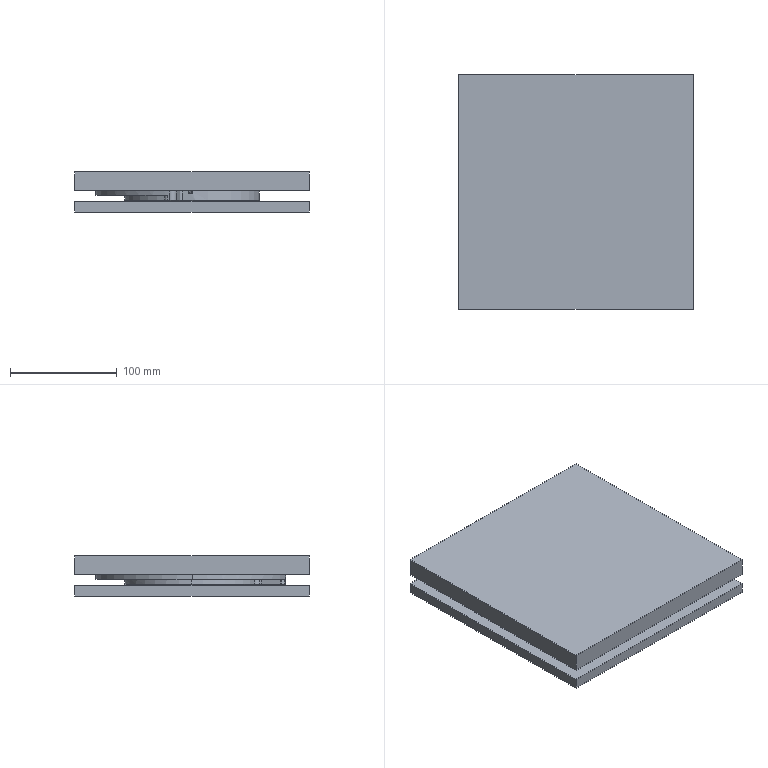NC program | NX | posted with a generic post | part box 220 x 220 x 37.5 mm
Lines 1 to 818 of 4969:
N10 G17 G21 G94 G90
(ADAPTIVE_MILLING_COPY_COPY , TOOL : D10)
N12 T03 M6
N14 G54
N16 G17 G0 G90 X-76.959 Y-29.515 S8000 M3
N18 G43 Z30. H3
N20 Z-4.5
N22 G94 G3 X-76.959 Y-29.515 Z-4.994 I2.51 J-3.735 F1000.
N24 X-76.959 Y-29.515 Z-5.487 I2.51 J-3.735
N26 X-76.959 Y-29.515 Z-5.981 I2.51 J-3.735
N28 X-76.959 Y-29.515 Z-6.474 I2.51 J-3.735
N30 X-76.959 Y-29.515 Z-6.968 I2.51 J-3.735
N32 X-76.959 Y-29.515 Z-7.461 I2.51 J-3.735
N34 X-76.959 Y-29.515 Z-7.955 I2.51 J-3.735
N36 X-76.959 Y-29.515 Z-8.448 I2.51 J-3.735
N38 X-76.959 Y-29.515 Z-8.942 I2.51 J-3.735
N40 X-76.959 Y-29.515 Z-9.435 I2.51 J-3.735
N42 X-76.959 Y-29.515 Z-9.929 I2.51 J-3.735
N44 X-76.959 Y-29.515 Z-10.422 I2.51 J-3.735
N46 X-76.959 Y-29.515 Z-10.916 I2.51 J-3.735
N48 X-76.959 Y-29.515 Z-11.409 I2.51 J-3.735
N50 X-76.959 Y-29.515 Z-11.903 I2.51 J-3.735
N52 X-74.448 Y-28.75 Z-12.35 R-4.5
N54 X-71.843 Y-29.571 R-4.501 F3500.
N56 X-79.316 Y-34.242 R4.669
N58 X-70.976 Y-29.663 R-4.977
N60 X-79.544 Y-35.212 R5.197
N62 X-70.592 Y-29.324 R-5.476
N64 X-80.049 Y-35.338 R5.713
N66 X-69.779 Y-29.447 R-5.996
N68 X-80.555 Y-35.529 R6.255
N70 X-69.211 Y-29.287 R-6.539
N72 X-81.051 Y-35.798 R6.811
N74 X-68.461 Y-29.383 R-7.099
N76 X-81.371 Y-36.522 R7.387
N78 X-67.943 Y-29.096 R-7.686
N80 X-82.268 Y-35.885 R7.977
N82 X-66.893 Y-29.789 R-8.279
N84 X-82.846 Y-36.084 R8.584
N86 X-66.106 Y-30.082 R-8.893
N88 X-83.638 Y-35.591 R9.201
N90 X-65.246 Y-30.689 R-9.518
N92 X-84.379 Y-35.214 R9.837
N94 X-64.383 Y-31.629 R10.159
N96 X-85.001 Y-35.455 R-10.488
N98 X-63.728 Y-31.519 R10.82
N100 X-85.867 Y-34.038 R11.152
N102 X-62.972 Y-32.124 R-11.489
N104 X-86.567 Y-33.269 R11.826
N106 X-62.238 Y-33.484 R12.165
N108 X-87.215 Y-32.245 R12.51
N110 X-61.613 Y-34.613 R12.856
N112 X-85.285 Y-25.329 R13.185
N114 X-87.451 Y-37.11 R13.203
N116 X-85.584 Y-40.924 R36.55
N118 X-69.729 Y-46.031 R13.403
N120 X-65.769 Y-43.648 R45.627
N122 X-61.177 Y-29.971 R13.404
N124 G2 X-62.905 Y-26.146 R61.413
N126 G3 X-71.532 Y-19.668 R12.951
N128 X-88.733 Y-33.803 R14.043
N130 G1 X-87.469 Y-37.067
N132 X-86.14 Y-39.947
N134 G3 X-84.694 Y-42.852 R21.488
N136 X-78.233 Y-47.097 R11.843
N138 X-72.577 Y-47.493 R14.192
N140 X-69.664 Y-45.994 R22.521
N142 X-69.806 Y-44.984 R0.551
N144 G1 X-70.024 Y-44.93
N146 X-71.965 Y-44.448 Z-12.25
N148 X-82.409 Y-41.859
N150 X-84.351 Y-41.378 Z-12.35
N152 G3 X-84.937 Y-41.406 R0.694
N154 X-85.144 Y-42.102 R0.554
N156 X-77.927 Y-47.901 R10.278
N158 X-72.58 Y-47.494 R10.689
N160 G1 X-72.466 Y-47.441
N162 G3 X-72.585 Y-46.404 R0.55
N164 G1 X-82.495 Y-44.345
N166 G3 X-82.929 Y-45.264 R0.551
N168 G1 X-82.791 Y-45.417
N170 X-82.716 Y-45.486
N172 X-81.828 Y-46.165
N174 G3 X-79.182 Y-47.535 R8.747
N176 G1 X-77.927 Y-47.901
N178 X-77.029 Y-48.003
N180 X-76.13 Y-48.091
N182 X-75.228 Y-48.03
N184 X-74.328 Y-47.953
N186 X-73.452 Y-47.731
N188 X-72.58 Y-47.494
N190 X-70.963 Y-46.744
N192 X-66.698 Y-44.281
N194 G3 X-63.932 Y-42.583 R22.347
N196 X-60.357 Y-36.135 R11.686
N198 X-60.112 Y-32.012 R13.658
N200 G1 X-61.211 Y-29.907
N202 G3 X-62.231 Y-30.024 R0.551
N204 G1 X-62.301 Y-30.296
N206 X-62.801 Y-32.232 Z-12.25
N208 X-64.895 Y-40.336
N210 X-65.395 Y-42.272 Z-12.35
N212 X-65.452 Y-42.501
N214 X-65.453 Y-42.736
N216 G3 X-64.641 Y-43.094 R0.551
N218 X-62.357 Y-41.58 R10.606
N220 X-59.502 Y-35.576 R11.215
N222 X-59.353 Y-33.465 R6.671
N224 G1 X-60.163 Y-31.914
N226 G3 X-61.178 Y-32.012 R0.551
N228 G1 X-61.239 Y-32.218
N230 X-61.808 Y-34.135 Z-12.25
N232 X-63.389 Y-39.468
N234 X-63.958 Y-41.386 Z-12.35
N236 X-64.023 Y-41.6
N238 X-64.058 Y-41.821
N240 G3 X-63.234 Y-42.281 R0.551
N242 X-61.017 Y-40.685 R7.564
N244 X-58.687 Y-34.729 R10.602
N246 X-59.189 Y-33.779 R2.823
N248 G1 X-59.363 Y-33.447
N250 G3 X-60.372 Y-33.527 R0.551
N252 G1 X-62.861 Y-41.03
N254 G3 X-62.043 Y-41.594 R0.551
N256 X-58.813 Y-38.102 R6.347
N258 X-58.176 Y-35.454 R5.89
N260 G1 X-58.211 Y-35.353
N262 X-58.805 Y-34.398
N264 G3 X-59.791 Y-34.505 R0.551
N266 G1 X-61.885 Y-40.458
N268 G3 X-61.068 Y-41.031 R0.551
N270 X-57.698 Y-36.382 R5.887
N272 G1 X-57.705 Y-36.258
N274 X-57.736 Y-36.137
N276 X-57.752 Y-36.091
N278 X-58.214 Y-35.348
N280 G3 X-59.194 Y-35.44 R0.551
N282 G1 X-60.908 Y-39.88
N284 G3 X-60.094 Y-40.469 R0.551
N286 X-57.388 Y-37.376 R4.939
N288 X-57.38 Y-36.689 R1.267
N290 G1 X-57.776 Y-36.052
N292 G3 X-58.754 Y-36.139 R0.551
N294 G1 X-60.04 Y-39.375
N296 G3 X-59.228 Y-39.969 R0.551
N298 X-57.418 Y-38.484 R4.401
N300 X-57.076 Y-37.193 R1.664
N302 G1 X-57.087 Y-37.161
N304 X-57.417 Y-36.63
N306 G3 X-58.401 Y-36.733 R0.551
N308 G1 X-59.178 Y-38.891
N310 G3 X-58.362 Y-39.469 R0.551
N312 X-56.922 Y-38.148 R2.881
N314 X-56.88 Y-37.494 R0.883
N316 G1 X-57.144 Y-37.07
N318 G3 X-58.138 Y-37.202 R0.551
N320 G1 X-58.533 Y-38.545
N322 G3 X-57.713 Y-39.094 R0.551
N324 X-56.699 Y-38.062 R1.712
N326 X-56.884 Y-37.487 R0.874
N328 X-57.871 Y-37.598 R0.551
N330 G1 X-58.097 Y-38.274
N332 G3 X-57.28 Y-38.844 R0.551
N334 X-56.62 Y-38.151 R1.03
N336 X-56.807 Y-37.612 R0.903
N338 X-57.817 Y-37.988 R0.55
N340 G1 X-57.783 Y-38.214
N342 X-57.718 Y-38.434
N344 G3 X-56.955 Y-38.656 R0.552
N346 X-56.662 Y-37.852 R0.583
N348 G1 X-59.189 Y-33.779
N350 X-61.558 Y-29.24
N352 X-62.743 Y-26.484
N354 G3 X-64.114 Y-23.548 R20.329
N356 X-70.254 Y-19.25 R11.851
N358 X-89.427 Y-31.954 R14.762
N360 G1 X-89.413 Y-32.044
N362 X-88.691 Y-33.91
N364 G3 X-88.036 Y-34.242 R0.554
N366 G1 X-86.162 Y-33.545 Z-12.25
N368 X-65.722 Y-25.908
N370 X-63.85 Y-25.205 Z-12.35
N372 G3 X-63.579 Y-24.536 R0.554
N374 X-64.724 Y-22.056 R7.534
N376 X-70.555 Y-18.382 R11.483
N378 X-89.96 Y-30.336 R15.473
N380 X-89.408 Y-32.059 R9.865
N382 X-88.751 Y-32.391 R0.554
N384 G1 X-86.861 Y-31.737 Z-12.25
N386 X-66.218 Y-24.576
N388 X-64.329 Y-23.92 Z-12.35
N390 G3 X-64.026 Y-23.236 R0.553
N392 X-66.919 Y-19.308 R6.494
N394 X-77.582 Y-17.26 R14.577
N396 X-90.396 Y-28.882 R16.145
N398 G1 X-90.399 Y-29.007
N400 X-90.394 Y-29.071
N402 X-89.942 Y-30.502
N404 G3 X-89.31 Y-30.876 R0.554
N406 G1 X-87.407 Y-30.26 Z-12.25
N408 X-66.596 Y-23.478
N410 X-64.696 Y-22.856 Z-12.35
N412 G3 X-64.392 Y-22.172 R0.553
N414 X-67.237 Y-18.369 R6.139
N416 X-76.833 Y-16.363 R14.504
N418 X-90.71 Y-27.344 R16.839
N420 X-90.781 Y-27.843 R3.366
N422 G1 X-90.367 Y-29.154
N424 G3 X-89.735 Y-29.528 R0.554
N426 G1 X-87.826 Y-28.933 Z-12.25
N428 X-66.969 Y-22.393
N430 X-65.061 Y-21.792 Z-12.35
N432 G3 X-64.757 Y-21.108 R0.553
N434 X-67.471 Y-17.513 R5.788
N436 X-75.969 Y-15.503 R14.213
N438 X-90.942 Y-25.844 R17.566
N440 X-91.142 Y-26.701 R2.262
N442 G1 X-90.765 Y-27.893
N444 G3 X-90.132 Y-28.267 R0.554
N446 G1 X-88.216 Y-27.695 Z-12.25
N448 X-67.302 Y-21.424
N450 X-65.387 Y-20.847 Z-12.35
N452 G3 X-65.082 Y-20.162 R0.553
N454 X-65.867 Y-18.343 R5.932
N456 X-70.182 Y-15.489 R8.932
N458 X-82.83 Y-16.479 R17.009
N460 X-91.201 Y-24.596 R17.861
N462 X-91.463 Y-25.68 R1.818
N464 G1 X-91.453 Y-25.714
N466 X-91.114 Y-26.787
N468 G3 X-90.48 Y-27.161 R0.554
N470 G1 X-88.556 Y-26.616 Z-12.25
N472 X-67.566 Y-20.654
N474 X-65.643 Y-20.106 Z-12.35
N476 G3 X-65.305 Y-19.452 R0.554
N478 X-67.529 Y-16.117 R4.962
N480 X-74.724 Y-13.937 R13.125
N482 X-91.36 Y-23.252 R18.728
N484 X-91.774 Y-24.419 R2.696
N486 G1 X-91.474 Y-25.633
N488 G3 X-90.834 Y-26.04 R0.553
N490 G1 X-88.903 Y-25.517 Z-12.25
N492 X-67.811 Y-19.79
N494 X-65.881 Y-19.265 Z-12.35
N496 G3 X-65.527 Y-18.605 R0.553
N498 X-67.766 Y-15.284 R4.928
N500 X-74.979 Y-13.159 R13.186
N502 X-91.477 Y-21.932 R19.338
N504 X-92.044 Y-23.326 R3.132
N506 G1 X-91.744 Y-24.54
N508 G3 X-91.137 Y-24.953 R0.554
N510 G1 X-89.201 Y-24.452 Z-12.25
N512 X-68.037 Y-18.925
N514 X-66.102 Y-18.418 Z-12.35
N516 G3 X-65.748 Y-17.759 R0.553
N518 X-68.01 Y-14.456 R4.877
N520 X-74.987 Y-12.385 R13.087
N522 X-91.623 Y-20.742 R19.839
N524 X-92.304 Y-22.204 R4.269
N526 G1 X-92.302 Y-22.279
N528 X-92.033 Y-23.372
N530 G3 X-91.425 Y-23.785 R0.554
N532 G1 X-89.483 Y-23.307 Z-12.25
N534 X-68.264 Y-18.054
N536 X-66.324 Y-17.572 Z-12.35
N538 G3 X-65.969 Y-16.912 R0.553
N540 X-68.152 Y-13.698 R4.798
N542 X-75.122 Y-11.611 R12.998
N544 X-91.598 Y-19.365 R20.468
N546 X-92.55 Y-21.111 R5.955
N548 X-92.284 Y-22.355 R6.523
N550 X-91.676 Y-22.768 R0.554
N552 G1 X-89.731 Y-22.303 Z-12.25
N554 X-68.489 Y-17.195
N556 X-66.545 Y-16.725 Z-12.35
N558 G3 X-66.191 Y-16.066 R0.553
N560 X-68.3 Y-12.945 R4.716
N562 X-74.762 Y-10.859 R12.562
N564 X-91.767 Y-18.315 R20.807
N566 X-92.797 Y-20.154 R5.347
N568 X-92.526 Y-21.374 R35.32
N570 X-91.918 Y-21.787 R0.554
N572 G1 X-89.968 Y-21.342 Z-12.25
N574 X-68.684 Y-16.451
N576 X-66.735 Y-16. Z-12.35
N578 G3 X-66.38 Y-15.34 R0.553
N580 X-68.439 Y-12.195 R4.628
N582 X-74.891 Y-10.083 R12.549
N584 X-91.999 Y-17.359 R21.134
N586 X-93.008 Y-19.073 R5.965
N588 X-92.783 Y-20.334 R5.638
N590 X-92.174 Y-20.747 R0.554
N592 G1 X-90.219 Y-20.323 Z-12.25
N594 X-68.888 Y-15.669
N596 X-66.935 Y-15.241 Z-12.35
N598 G3 X-66.559 Y-14.617 R0.554
N600 X-68.367 Y-11.601 R4.275
N602 X-74.385 Y-9.367 R11.921
N604 X-87.846 Y-12.695 R21.193
N606 X-92.728 Y-17.108 R16.692
N608 X-93.207 Y-18.169 R2.453
N610 G1 X-93.007 Y-19.276
N612 G3 X-92.425 Y-19.727 R0.554
N614 G1 X-90.466 Y-19.328 Z-12.25
N616 X-69.056 Y-14.915
N618 X-67.097 Y-14.511 Z-12.35
N620 G3 X-66.694 Y-13.88 R0.553
N622 X-68.493 Y-10.856 R4.293
N624 X-74.376 Y-8.61 R11.794
N626 X-87.35 Y-11.424 R21.302
N628 X-92.793 Y-15.945 R17.496
N630 X-93.388 Y-17.165 R2.508
N632 G1 X-93.188 Y-18.272
N634 G3 X-92.609 Y-18.723 R0.554
N636 G1 X-90.645 Y-18.344 Z-12.25
N638 X-69.194 Y-14.157
N640 X-67.231 Y-13.773 Z-12.35
N642 G3 X-66.828 Y-13.142 R0.553
N644 X-68.611 Y-10.107 R4.318
N646 X-74.733 Y-7.804 R12.003
N648 X-88.032 Y-10.85 R21.836
N650 X-93.061 Y-15.094 R16.446
N652 X-93.567 Y-16.172 R2.304
N654 G1 X-93.367 Y-17.279
N656 G3 X-92.788 Y-17.73 R0.554
N658 G1 X-90.82 Y-17.37 Z-12.25
N660 X-69.332 Y-13.4
N662 X-67.366 Y-13.035 Z-12.35
N664 G3 X-66.963 Y-12.404 R0.553
N666 X-68.827 Y-9.282 R4.373
N668 X-75.089 Y-7. R12.255
N670 X-88.063 Y-9.897 R22.221
N672 X-93.097 Y-13.945 R16.752
N674 X-93.743 Y-15.199 R2.616
N676 G1 X-93.565 Y-16.183
N678 G3 X-92.985 Y-16.634 R0.554
N680 G1 X-91.013 Y-16.301 Z-12.25
N682 X-69.472 Y-12.635
N684 X-67.5 Y-12.297 Z-12.35
N686 G3 X-67.098 Y-11.666 R0.553
N688 X-68.947 Y-8.533 R4.412
N690 X-74.949 Y-6.248 R12.117
N692 X-87.536 Y-8.66 R22.256
N694 X-93.118 Y-12.808 R17.79
N696 X-93.914 Y-14.203 R3.167
N698 G1 X-93.915 Y-14.242
N700 X-93.738 Y-15.226
N702 G3 X-93.157 Y-15.677 R0.554
N704 G1 X-91.182 Y-15.361 Z-12.25
N706 X-69.609 Y-11.88
N708 X-67.635 Y-11.559 Z-12.35
N710 G3 X-67.232 Y-10.928 R0.553
N712 X-69.064 Y-7.785 R4.412
N714 X-75.178 Y-5.453 R12.178
N716 X-87.888 Y-7.892 R22.628
N718 X-93.364 Y-11.971 R17.075
N720 X-94.059 Y-13.197 R2.821
N722 G1 X-93.982 Y-13.868
N724 X-93.977 Y-13.903
N726 X-93.91 Y-14.272
N728 G3 X-93.328 Y-14.723 R0.554
N730 G1 X-91.351 Y-14.423 Z-12.25
N732 X-69.747 Y-11.126
N734 X-67.77 Y-10.822 Z-12.35
N736 G3 X-67.367 Y-10.19 R0.553
N738 X-69.074 Y-7.12 R4.279
N740 X-75.022 Y-4.706 R11.95
N742 X-87.211 Y-6.636 R22.517
N744 X-93.277 Y-10.745 R18.617
N746 X-94.167 Y-12.088 R4.189
N748 G1 X-94.177 Y-12.177
N750 X-94.048 Y-13.295
N752 G3 X-93.498 Y-13.782 R0.554
N754 G1 X-91.517 Y-13.507 Z-12.25
N756 X-69.871 Y-10.454
N758 X-67.891 Y-10.173 Z-12.35
N760 G3 X-67.468 Y-9.579 R0.554
N762 X-68.981 Y-6.542 R4.073
N764 X-74.733 Y-3.989 R11.493
N766 X-86.734 Y-5.514 R22.321
N768 X-93.33 Y-9.712 R19.103
N770 X-94.287 Y-11.152 R3.369
N772 G1 X-94.291 Y-11.187
N774 X-94.177 Y-12.18
N776 G3 X-93.627 Y-12.667 R0.554
N778 G1 X-91.642 Y-12.42 Z-12.25
N780 X-69.981 Y-9.684
N782 X-67.997 Y-9.433 Z-12.35
N784 G3 X-67.547 Y-8.833 R0.553
N786 X-69.068 Y-5.798 R4.118
N788 X-74.561 Y-3.26 R11.361
N790 X-86.354 Y-4.459 R22.14
N792 X-93.197 Y-8.502 R20.134
N794 X-94.386 Y-10.09 R5.034
N796 X-94.288 Y-11.215 R14.31
N798 X-93.738 Y-11.702 R0.554
N800 G1 X-91.75 Y-11.481 Z-12.25
N802 X-70.049 Y-9.036
N804 X-68.062 Y-8.811 Z-12.35
N806 G3 X-67.613 Y-8.212 R0.553
N808 X-69.241 Y-4.965 R4.289
N810 X-74.998 Y-2.413 R11.816
N812 X-87.251 Y-3.9 R22.68
N814 X-93.492 Y-7.74 R18.787
N816 X-94.501 Y-9.151 R4.324
N818 G1 X-94.513 Y-9.261
N820 X-94.399 Y-10.254
N822 G3 X-93.848 Y-10.741 R0.554
N824 G1 X-91.859 Y-10.536 Z-12.25
N826 X-70.13 Y-8.274
N828 X-68.141 Y-8.065 Z-12.35
N830 G3 X-67.692 Y-7.466 R0.553
N832 X-69.317 Y-4.217 R4.3
N834 X-75.061 Y-1.633 R11.874
N836 X-86.978 Y-2.885 R22.734
N838 X-93.512 Y-6.715 R19.066
N840 X-94.612 Y-8.211 R4.22
N842 G1 X-94.623 Y-8.309
N844 X-94.509 Y-9.303
N846 G3 X-93.957 Y-9.79 R0.554
N848 G1 X-91.966 Y-9.6 Z-12.25
N850 X-70.21 Y-7.512
N852 X-68.22 Y-7.319 Z-12.35
N854 G3 X-67.771 Y-6.72 R0.553
N856 X-69.391 Y-3.467 R4.323
N858 X-75.244 Y-0.828 R12.04
N860 X-87.635 Y-2.228 R23.143
N862 X-93.793 Y-5.958 R17.855
N864 X-94.703 Y-7.286 R2.976
N866 G1 X-94.673 Y-7.865
N868 X-94.67 Y-7.901
N870 X-94.613 Y-8.398
N872 G3 X-94.061 Y-8.885 R0.554
N874 G1 X-92.069 Y-8.708 Z-12.25
N876 X-70.291 Y-6.754
N878 X-68.299 Y-6.573 Z-12.35
N880 G3 X-67.85 Y-5.974 R0.553
N882 X-69.462 Y-2.717 R4.335
N884 X-75.3 Y-0.045 R12.025
N886 X-87.587 Y-1.299 R23.226
N888 X-93.803 Y-4.936 R18.29
N890 X-94.755 Y-6.266 R3.047
N892 G1 X-94.698 Y-7.39
N894 G3 X-94.174 Y-7.911 R0.554
N896 G1 X-92.18 Y-7.754 Z-12.25
N898 X-70.372 Y-5.992
N900 X-68.379 Y-5.828 Z-12.35
N902 G3 X-67.929 Y-5.229 R0.553
N904 X-69.521 Y-1.966 R4.338
N906 X-75.223 Y0.714 R12.051
N908 X-87.643 Y-0.417 R23.247
N910 X-93.799 Y-3.913 R18.278
N912 X-94.789 Y-5.185 R4.096
N914 G1 X-94.806 Y-5.28
N916 X-94.755 Y-6.279
N918 G3 X-94.237 Y-6.8 R0.554
N920 G1 X-92.241 Y-6.678 Z-12.25
N922 X-70.445 Y-5.3
N924 X-68.45 Y-5.171 Z-12.35
N926 G3 X-67.993 Y-4.612 R0.554
N928 X-69.297 Y-1.484 R3.993
N930 X-74.643 Y1.351 R11.33
N932 X-86.132 Y0.961 R22.475
N934 X-93.491 Y-2.641 R20.316
N936 X-94.812 Y-4.126 R5.666
N938 X-94.805 Y-5.304 R4.11
N940 X-94.287 Y-5.825 R0.554
N942 G1 X-92.29 Y-5.719 Z-12.25
N944 X-70.506 Y-4.535
N946 X-68.509 Y-4.426 Z-12.35
N948 G3 X-68.016 Y-3.862 R0.553
N950 X-69.336 Y-0.736 R4.081
N952 X-74.787 Y2.161 R11.508
N954 X-86.16 Y1.836 R22.684
N956 X-93.55 Y-1.704 R20.399
N958 X-94.867 Y-3.189 R5.242
N960 X-94.854 Y-4.351 R4.711
N962 X-94.335 Y-4.871 R0.554
N964 G1 X-92.337 Y-4.791 Z-12.25
N966 X-70.526 Y-3.885
N968 X-68.527 Y-3.801 Z-12.35
N970 G3 X-68.035 Y-3.238 R0.553
N972 X-69.368 Y0.01 R4.144
N974 X-75.166 Y3.031 R11.827
N976 X-87.26 Y2.401 R23.356
N978 X-93.789 Y-0.925 R18.764
N980 X-94.918 Y-2.248 R4.993
N982 X-94.902 Y-3.403 R5.053
N984 X-94.383 Y-3.924 R0.554
N986 G1 X-92.384 Y-3.859 Z-12.25
N988 X-70.549 Y-3.121
N990 X-68.55 Y-3.052 Z-12.35
N992 G3 X-68.058 Y-2.488 R0.553
N994 X-69.394 Y0.761 R4.194
N996 X-74.934 Y3.754 R11.757
N998 X-86.555 Y3.49 R23.128
N1000 X-93.735 Y0.09 R19.519
N1002 X-94.958 Y-1.31 R4.498
N1004 X-94.949 Y-2.491 R33.287
N1006 X-94.429 Y-3.012 R0.554
N1008 G1 X-92.43 Y-2.959 Z-12.25
N1010 X-70.572 Y-2.359
N1012 X-68.573 Y-2.302 Z-12.35
N1014 G3 X-68.08 Y-1.738 R0.553
N1016 X-69.418 Y1.512 R4.231
N1018 X-74.941 Y4.537 R11.816
N1020 X-86.686 Y4.334 R23.211
N1022 X-93.672 Y1.099 R19.356
N1024 X-94.935 Y-0.267 R4.893
N1026 G1 X-94.964 Y-0.387
N1028 X-94.976 Y-1.387
N1030 G3 X-94.484 Y-1.94 R0.554
N1032 G1 X-92.485 Y-1.914 Z-12.25
N1034 X-70.596 Y-1.585
N1036 X-68.597 Y-1.553 Z-12.35
N1038 G3 X-68.103 Y-0.989 R0.553
N1040 X-69.437 Y2.265 R4.248
N1042 X-75.064 Y5.354 R11.959
N1044 X-86.811 Y5.181 R23.424
N1046 X-93.702 Y2.033 R19.314
N1048 X-94.94 Y0.654 R3.704
N1050 G1 X-94.952 Y0.606
N1052 X-94.964 Y-0.394
N1054 G3 X-94.48 Y-0.946 R0.554
N1056 G1 X-92.481 Y-0.939 Z-12.25
N1058 X-70.62 Y-0.817
N1060 X-68.62 Y-0.803 Z-12.35
N1062 G3 X-68.126 Y-0.239 R0.553
N1064 X-69.439 Y3.005 R4.238
N1066 X-74.924 Y6.1 R11.875
N1068 X-86.671 Y6.094 R23.317
N1070 X-93.709 Y2.974 R19.204
N1072 X-94.903 Y1.712 R4.728
N1074 X-94.952 Y0.577 R8.175
N1076 X-94.468 Y0.024 R0.554
N1078 G1 X-92.468 Y0.016 Z-12.25
N1080 X-70.643 Y-0.029
N1082 X-68.644 Y-0.03 Z-12.35
N1084 G3 X-68.148 Y0.493 R0.554
N1086 X-69.19 Y3.47 R3.847
N1088 X-74.188 Y6.656 R11.132
N1090 X-85.304 Y7.253 R22.457
N1092 X-93.308 Y4.205 R20.969
N1094 X-94.9 Y2.644 R5.076
N1096 G1 X-94.928 Y2.526
N1098 X-94.94 Y1.526
N1100 G3 X-94.456 Y0.974 R0.554
N1102 G1 X-92.457 Y0.932 Z-12.25
N1104 X-70.658 Y0.506
N1106 X-68.658 Y0.467 Z-12.35
N1108 G3 X-68.126 Y0.992 R0.553
N1110 X-69.176 Y4.216 R4.005
N1112 X-74.392 Y7.513 R11.367
N1114 X-85.759 Y8.03 R22.8
N1116 X-93.4 Y5.07 R20.315
N1118 X-94.89 Y3.585 R4.699
N1120 G1 X-94.916 Y3.476
N1122 X-94.929 Y2.476
N1124 G3 X-94.444 Y1.923 R0.554
N1126 G1 X-92.445 Y1.866 Z-12.25
N1128 X-70.625 Y1.27
N1130 X-68.626 Y1.216 Z-12.35
N1132 G3 X-68.092 Y1.742 R0.553
N1134 X-69.235 Y5.06 R4.127
N1136 X-74.472 Y8.331 R11.625
N1138 X-86.085 Y8.834 R23.081
N1140 X-93.483 Y5.936 R19.777
N1142 X-94.872 Y4.525 R4.148
N1144 G1 X-94.886 Y4.48
N1146 X-94.906 Y4.21
N1148 X-94.908 Y4.174
N1150 X-94.917 Y3.424
N1152 G3 X-94.431 Y2.871 R0.554
N1154 G1 X-92.433 Y2.79 Z-12.25
N1156 X-70.596 Y1.919
N1158 X-68.598 Y1.841 Z-12.35
N1160 G3 X-68.064 Y2.366 R0.553
N1162 X-69.209 Y5.809 R4.222
N1164 X-74.546 Y9.151 R11.817
N1166 X-86.527 Y9.614 R23.401
N1168 X-93.456 Y6.868 R19.223
N1170 X-94.785 Y5.57 R4.335
N1172 G1 X-94.809 Y5.492
N1174 X-94.894 Y4.37
N1176 G3 X-94.421 Y3.784 R0.553
N1178 G1 X-92.423 Y3.689 Z-12.25
N1180 X-70.563 Y2.681
N1182 X-68.565 Y2.59 Z-12.35
N1184 G3 X-68.031 Y3.115 R0.553
N1186 X-69.177 Y6.559 R4.254
N1188 X-74.496 Y9.933 R11.925
N1190 X-86.596 Y10.47 R23.563
N1192 X-93.421 Y7.801 R18.893
N1194 X-94.686 Y6.609 R4.91
N1196 X-94.81 Y5.475 R6.781
N1198 X-94.362 Y4.892 R0.554
N1200 G1 X-92.366 Y4.768 Z-12.25
N1202 X-70.528 Y3.457
N1204 X-68.531 Y3.339 Z-12.35
N1206 G3 X-67.997 Y3.864 R0.553
N1208 X-69.142 Y7.311 R4.285
N1210 X-74.56 Y10.757 R12.061
N1212 X-87.028 Y11.246 R23.752
N1214 X-93.588 Y8.588 R17.905
N1216 X-94.633 Y7.53 R3.756
N1218 G1 X-94.66 Y7.441
N1220 X-94.736 Y6.444
N1222 G3 X-94.289 Y5.861 R0.554
N1224 G1 X-92.294 Y5.721 Z-12.25
N1226 X-70.493 Y4.223
N1228 X-68.498 Y4.089 Z-12.35
N1230 G3 X-67.963 Y4.614 R0.553
N1232 X-69.104 Y8.063 R4.311
N1234 X-74.384 Y11.501 R12.08
N1236 X-86.721 Y12.179 R23.716
N1238 X-93.336 Y9.657 R18.089
N1240 X-94.572 Y8.447 R3.425
N1242 G1 X-94.588 Y8.397
N1244 X-94.663 Y7.4
N1246 G3 X-94.215 Y6.817 R0.554
N1248 G1 X-92.222 Y6.661 Z-12.25
N1250 X-70.459 Y4.988
N1252 X-68.465 Y4.838 Z-12.35
N1254 G3 X-67.93 Y5.363 R0.553
N1256 X-68.827 Y8.521 R4.033
N1258 X-73.969 Y12.151 R11.517
N1260 X-85.542 Y13.243 R23.148
N1262 X-92.971 Y10.791 R19.825
N1264 X-94.465 Y9.485 R4.993
N1266 X-94.591 Y8.345 R5.919
N1268 X-94.143 Y7.763 R0.554
N1270 G1 X-92.152 Y7.576 Z-12.25
N1272 X-70.433 Y5.567
N1274 X-68.441 Y5.384 Z-12.35
N1276 G3 X-67.888 Y5.868 R0.554
N1278 X-68.688 Y9.163 R4.013
N1280 X-73.649 Y12.832 R11.337
N1282 X-84.948 Y14.177 R22.897
N1284 X-92.787 Y11.79 R20.404
N1286 X-94.392 Y10.423 R5.232
N1288 X-94.517 Y9.326 R6.795
N1290 X-94.067 Y8.744 R0.554
N1292 G1 X-92.078 Y8.54 Z-12.25
N1294 X-70.359 Y6.331
N1296 X-68.369 Y6.129 Z-12.35
N1298 G3 X-67.798 Y6.613 R0.553
N1300 X-68.612 Y9.906 R4.06
N1302 X-73.553 Y13.604 R11.417
N1304 X-84.717 Y15.058 R22.841
N1306 X-92.589 Y12.782 R20.547
N1308 X-94.235 Y11.462 R5.694
N1310 X-94.447 Y10.235 R6.787
N1312 X-94. Y9.635 R0.553
N1314 G1 X-92.011 Y9.42 Z-12.25
N1316 X-70.268 Y7.086
N1318 X-68.279 Y6.874 Z-12.35
N1320 G3 X-67.708 Y7.358 R0.553
N1322 X-68.53 Y10.651 R4.101
N1324 X-73.452 Y14.378 R11.496
N1326 X-84.976 Y15.885 R23.01
N1328 X-92.492 Y13.709 R20.027
N1330 X-94.126 Y12.384 R4.54
N1332 G1 X-94.155 Y12.306
N1334 X-94.295 Y11.316
N1336 G3 X-93.885 Y10.706 R0.554
N1338 G1 X-91.901 Y10.454 Z-12.25
N1340 X-70.19 Y7.741
N1342 X-68.205 Y7.494 Z-12.35
N1344 G3 X-67.633 Y7.978 R0.553
N1346 X-68.515 Y11.5 R4.261
N1348 X-73.459 Y15.202 R11.757
N1350 X-85.106 Y16.726 R23.23
N1352 X-92.499 Y14.577 R19.631
N1354 X-93.956 Y13.416 R5.194
N1356 X-94.159 Y12.279 R5.061
N1358 X-93.75 Y11.669 R0.554
N1360 G1 X-91.768 Y11.4 Z-12.25
N1362 X-70.098 Y8.502
N1364 X-68.115 Y8.239 Z-12.35
N1366 G3 X-67.543 Y8.723 R0.553
N1368 X-68.423 Y12.246 R4.294
N1370 X-73.575 Y16.079 R12.057
N1372 X-85.603 Y17.523 R23.677
N1374 X-92.604 Y15.372 R18.187
N1376 X-93.84 Y14.336 R4.217
N1378 X-94.026 Y13.225 R23.169
N1380 X-93.616 Y12.616 R0.554
N1382 G1 X-91.637 Y12.332 Z-12.25
N1384 X-70.006 Y9.262
N1386 X-68.026 Y8.984 Z-12.35
N1388 G3 X-67.454 Y9.467 R0.553
N1390 X-68.329 Y12.993 R4.312
N1392 X-73.459 Y16.856 R12.088
N1394 X-85.351 Y18.411 R23.703
N1396 X-92.491 Y16.295 R18.229
N1398 X-93.719 Y15.253 R3.876
N1400 G1 X-93.755 Y15.158
N1402 X-93.894 Y14.168
N1404 G3 X-93.484 Y13.558 R0.554
N1406 G1 X-91.506 Y13.259 Z-12.25
N1408 X-69.914 Y10.022
N1410 X-67.936 Y9.728 Z-12.35
N1412 G3 X-67.364 Y10.212 R0.553
N1414 X-68.154 Y13.63 R4.203
N1416 X-73.216 Y17.579 R11.949
N1418 X-84.961 Y19.305 R23.583
N1420 X-92.148 Y17.343 R18.744
N1422 X-93.591 Y16.176 R4.038
N1424 G1 X-93.624 Y16.088
N1426 X-93.763 Y15.097
N1428 G3 X-93.352 Y14.487 R0.554
N1430 G1 X-91.378 Y14.167 Z-12.25
N1432 X-69.833 Y10.699
N1434 X-67.858 Y10.383 Z-12.35
N1436 G3 X-67.28 Y10.826 R0.554
N1438 X-67.832 Y14.051 R3.931
N1440 X-72.508 Y18.077 R11.345
N1442 X-83.554 Y20.25 R22.82
N1444 X-91.672 Y18.443 R20.356
N1446 X-93.379 Y17.209 R5.004
N1448 G1 X-93.419 Y17.121
N1450 X-93.605 Y16.218
N1452 X-93.611 Y16.182
N1454 X-93.628 Y16.059
N1456 G3 X-93.216 Y15.448 R0.554
N1458 G1 X-91.246 Y15.103 Z-12.25
N1460 X-69.735 Y11.343
N1462 X-67.764 Y10.999 Z-12.35
N1464 G3 X-67.159 Y11.439 R0.553
N1466 X-67.77 Y14.892 R4.086
N1468 X-72.581 Y18.954 R11.703
N1470 X-83.635 Y21.1 R23.128
N1472 X-91.403 Y19.418 R20.278
N1474 X-93.148 Y18.231 R5.556
N1476 X-93.42 Y17.114 R5.556
N1478 X-93.05 Y16.48 R0.554
N1480 G1 X-91.085 Y16.109 Z-12.25
N1482 X-69.586 Y12.101
N1484 X-67.62 Y11.735 Z-12.35
N1486 G3 X-67.014 Y12.175 R0.553
N1488 X-67.572 Y15.522 R4.081
N1490 X-72.423 Y19.721 R11.709
N1492 X-84.085 Y21.93 R23.435
N1494 X-91.579 Y20.172 R19.045
N1496 X-92.977 Y19.145 R4.316
N1498 G1 X-93.022 Y19.045
N1500 X-93.224 Y18.066
N1502 G3 X-92.854 Y17.431 R0.554
N1504 G1 X-90.894 Y17.035 Z-12.25
N1506 X-69.46 Y12.74
N1508 X-67.499 Y12.348 Z-12.35
N1510 G3 X-66.893 Y12.788 R0.553
N1512 X-67.497 Y16.365 R4.229
N1514 X-72.259 Y20.486 R11.784
N1516 X-83.653 Y22.802 R23.422
N1518 X-91.185 Y21.201 R19.65
N1520 X-92.797 Y20.055 R4.066
N1522 G1 X-92.828 Y19.987
N1524 X-93.03 Y19.008
N1526 G3 X-92.66 Y18.373 R0.554
N1528 G1 X-90.703 Y17.961 Z-12.25
N1530 X-69.312 Y13.491
N1532 X-67.354 Y13.084 Z-12.35
N1534 G3 X-66.748 Y13.524 R0.553
N1536 X-67.352 Y17.104 R4.278
N1538 X-71.981 Y21.193 R11.805
N1540 X-83.592 Y23.655 R23.43
N1542 X-91.01 Y22.116 R19.444
N1544 X-92.554 Y21.073 R5.163
N1546 X-92.838 Y19.938 R4.328
N1548 X-92.468 Y19.303 R0.554
N1550 G1 X-90.514 Y18.877 Z-12.25
N1552 X-69.164 Y14.242
N1554 X-67.209 Y13.82 Z-12.35
N1556 G3 X-66.602 Y14.259 R0.553
N1558 X-67.202 Y17.843 R4.309
N1560 X-72.031 Y22.075 R12.038
N1562 X-84.151 Y24.481 R23.786
N1564 X-91.054 Y22.913 R17.967
N1566 X-92.432 Y21.871 R3.179
N1568 G1 X-92.447 Y21.837
N1570 X-92.649 Y20.858
N1572 G3 X-92.278 Y20.223 R0.554
N1574 G1 X-90.327 Y19.782 Z-12.25
N1576 X-69.016 Y14.992
N1578 X-67.064 Y14.556 Z-12.35
N1580 G3 X-66.457 Y14.995 R0.553
N1582 X-67.019 Y18.531 R4.294
N1584 X-71.913 Y22.874 R12.208
N1586 X-84.148 Y25.332 R23.946
N1588 X-90.928 Y23.79 R17.474
N1590 X-92.143 Y22.929 R4.429
N1592 G1 X-92.194 Y22.834
N1594 X-92.385 Y22.135
N1596 X-92.393 Y22.1
N1598 X-92.469 Y21.733
N1600 G3 X-92.097 Y21.098 R0.554
N1602 G1 X-90.149 Y20.645 Z-12.25
N1604 X-68.871 Y15.723
N1606 X-66.922 Y15.275 Z-12.35
N1608 G3 X-66.322 Y15.675 R0.554
N1610 X-66.671 Y18.927 R3.912
N1612 X-70.954 Y23.198 R11.222
N1614 X-81.928 Y26.204 R22.767
N1616 X-90.036 Y25.013 R20.502
N1618 X-91.85 Y23.935 R5.676
N1620 X-92.226 Y22.715 R6.088
N1622 X-91.897 Y22.058 R0.554
N1624 G1 X-89.956 Y21.576 Z-12.25
N1626 X-68.736 Y16.361
N1628 X-66.794 Y15.884 Z-12.35
N1630 G3 X-66.156 Y16.277 R0.553
N1632 X-66.488 Y19.652 R4.039
N1634 X-70.856 Y24.013 R11.465